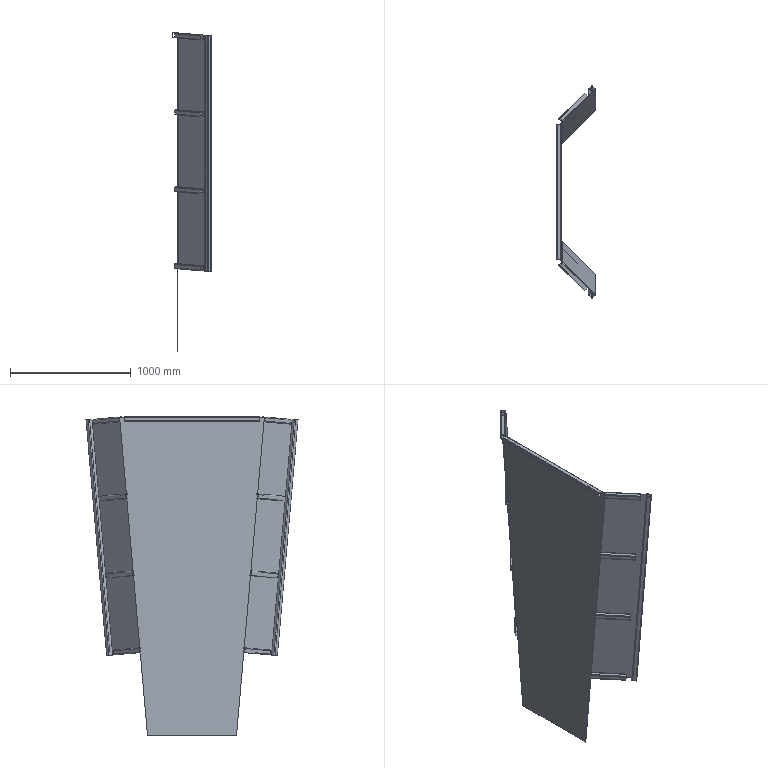Part | STEP file | COMPOUND | 14 solids | 216 faces | box 325.47 x 1761 x 2643 mm | volume 11287286 mm3 | plane 128 | cylinder 88 | commonest cylinder face diameters 6 x44 12 x44